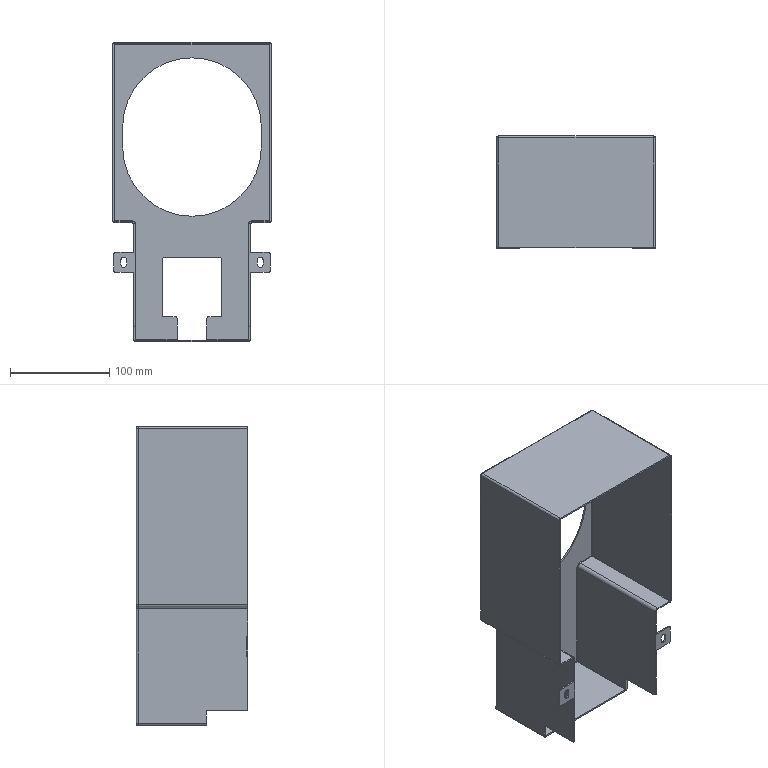Part | STEP file | ND25021-01-JDKM-08-BJ | 1 solid | 115 faces | box 160 x 113 x 302 mm | volume 174803 mm3 | cylinder 55 | plane 44 | sphere 12 | torus 4 | commonest cylinder face diameters 4 x29 1 x15 6 x6 140 x3 7 x2